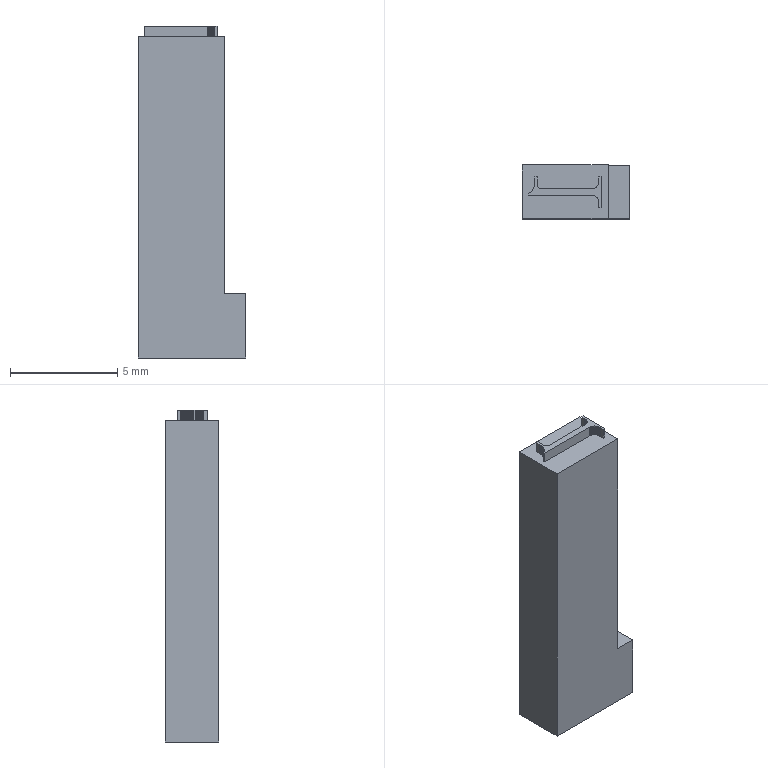Part | NX | features DIE-33 2 | 1 solid | 83 faces | box 5 x 2.5 x 15.5 mm | volume 158.142 mm3 | plane 83